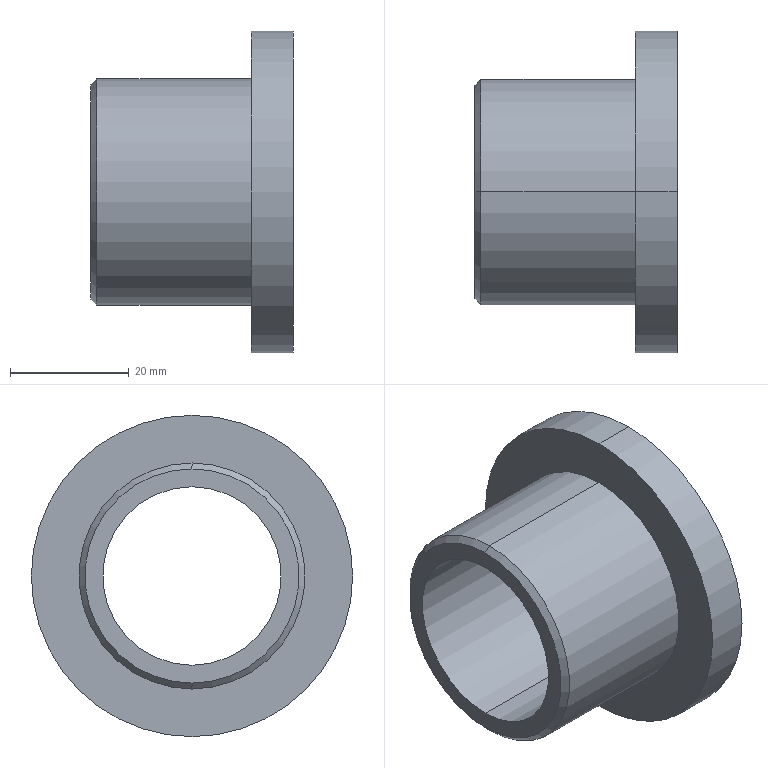Part | SolidWorks | features Chamfer 1, Revolution 1 | 1 solid | 11 faces | box 34 x 54 x 54 mm | volume 22561 mm3 | cylinder 6 | plane 3 | cone 2 | commonest cylinder face diameters 30 x2 38 x2 54 x2
STEP:
#1=CARTESIAN_POINT('',(0.,0.,18.));
#2=VERTEX_POINT('',#1);
#3=CARTESIAN_POINT('',(0.,0.,-18.));
#4=VERTEX_POINT('',#3);
#5=CARTESIAN_POINT('',(0.,0.,0.));
#6=DIRECTION('',(-1.,0.,0.));
#7=DIRECTION('',(0.,0.,-1.));
#8=AXIS2_PLACEMENT_3D('',#5,#6,#7);
#9=CIRCLE('',#8,18.);
#10=EDGE_CURVE('',#2,#4,#9,.T.);
#11=ORIENTED_EDGE('',*,*,#10,.F.);
#12=CARTESIAN_POINT('',(1.,0.,19.));
#13=VERTEX_POINT('',#12);
#14=CARTESIAN_POINT('',(0.,0.,18.));
#15=DIRECTION('',(0.7071,0.,0.7071));
#16=VECTOR('',#15,1000.);
#17=LINE('',#14,#16);
#18=EDGE_CURVE('',#2,#13,#17,.T.);
#19=ORIENTED_EDGE('',*,*,#18,.T.);
#20=CARTESIAN_POINT('',(1.,0.,-19.));
#21=VERTEX_POINT('',#20);
#22=CARTESIAN_POINT('',(1.,0.,0.));
#23=DIRECTION('',(1.,0.,0.));
#24=DIRECTION('',(0.,0.,-1.));
#25=AXIS2_PLACEMENT_3D('',#22,#23,#24);
#26=CIRCLE('',#25,19.);
#27=EDGE_CURVE('',#21,#13,#26,.T.);
#28=ORIENTED_EDGE('',*,*,#27,.F.);
#29=CARTESIAN_POINT('',(0.,0.,-18.));
#30=DIRECTION('',(0.7071,0.,-0.7071));
#31=VECTOR('',#30,1000.);
#32=LINE('',#29,#31);
#33=EDGE_CURVE('',#4,#21,#32,.T.);
#34=ORIENTED_EDGE('',*,*,#33,.F.);
#35=EDGE_LOOP('',(#11,#19,#28,#34));
#36=FACE_OUTER_BOUND('',#35,.T.);
#37=CARTESIAN_POINT('',(0.,0.,0.));
#38=DIRECTION('',(1.,0.,0.));
#39=DIRECTION('',(0.,0.,-1.));
#40=AXIS2_PLACEMENT_3D('',#37,#38,#39);
#41=CONICAL_SURFACE('',#40,18.,0.7854);
#42=ADVANCED_FACE('',(#36),#41,.T.);
#43=CARTESIAN_POINT('',(27.,0.,19.));
#44=VERTEX_POINT('',#43);
#45=CARTESIAN_POINT('',(27.,0.,-19.));
#46=VERTEX_POINT('',#45);
#47=CARTESIAN_POINT('',(27.,0.,0.));
#48=DIRECTION('',(-1.,0.,0.));
#49=DIRECTION('',(0.,0.,1.));
#50=AXIS2_PLACEMENT_3D('',#47,#48,#49);
#51=CIRCLE('',#50,19.);
#52=EDGE_CURVE('',#44,#46,#51,.T.);
#53=ORIENTED_EDGE('',*,*,#52,.T.);
#54=CARTESIAN_POINT('',(0.,0.,-19.));
#55=DIRECTION('',(-1.,0.,0.));
#56=VECTOR('',#55,1000.);
#57=LINE('',#54,#56);
#58=EDGE_CURVE('',#46,#21,#57,.T.);
#59=ORIENTED_EDGE('',*,*,#58,.T.);
#60=ORIENTED_EDGE('',*,*,#27,.T.);
#61=CARTESIAN_POINT('',(0.,0.,19.));
#62=DIRECTION('',(-1.,0.,0.));
#63=VECTOR('',#62,1000.);
#64=LINE('',#61,#63);
#65=EDGE_CURVE('',#44,#13,#64,.T.);
#66=ORIENTED_EDGE('',*,*,#65,.F.);
#67=EDGE_LOOP('',(#53,#59,#60,#66));
#68=FACE_OUTER_BOUND('',#67,.T.);
#69=CARTESIAN_POINT('',(0.,0.,0.));
#70=DIRECTION('',(-1.,0.,0.));
#71=DIRECTION('',(0.,0.,1.));
#72=AXIS2_PLACEMENT_3D('',#69,#70,#71);
#73=CYLINDRICAL_SURFACE('',#72,19.);
#74=ADVANCED_FACE('',(#68),#73,.T.);
#75=CARTESIAN_POINT('',(34.,0.,27.));
#76=VERTEX_POINT('',#75);
#77=CARTESIAN_POINT('',(34.,0.,-27.));
#78=VERTEX_POINT('',#77);
#79=CARTESIAN_POINT('',(34.,0.,0.));
#80=DIRECTION('',(-1.,0.,0.));
#81=DIRECTION('',(0.,0.,1.));
#82=AXIS2_PLACEMENT_3D('',#79,#80,#81);
#83=CIRCLE('',#82,27.);
#84=EDGE_CURVE('',#76,#78,#83,.T.);
#85=ORIENTED_EDGE('',*,*,#84,.T.);
#86=CARTESIAN_POINT('',(27.,0.,-27.));
#87=VERTEX_POINT('',#86);
#88=CARTESIAN_POINT('',(0.,0.,-27.));
#89=DIRECTION('',(-1.,0.,0.));
#90=VECTOR('',#89,1000.);
#91=LINE('',#88,#90);
#92=EDGE_CURVE('',#78,#87,#91,.T.);
#93=ORIENTED_EDGE('',*,*,#92,.T.);
#94=CARTESIAN_POINT('',(27.,0.,27.));
#95=VERTEX_POINT('',#94);
#96=CARTESIAN_POINT('',(27.,0.,0.));
#97=DIRECTION('',(-1.,0.,0.));
#98=DIRECTION('',(0.,0.,1.));
#99=AXIS2_PLACEMENT_3D('',#96,#97,#98);
#100=CIRCLE('',#99,27.);
#101=EDGE_CURVE('',#95,#87,#100,.T.);
#102=ORIENTED_EDGE('',*,*,#101,.F.);
#103=CARTESIAN_POINT('',(0.,0.,27.));
#104=DIRECTION('',(-1.,0.,0.));
#105=VECTOR('',#104,1000.);
#106=LINE('',#103,#105);
#107=EDGE_CURVE('',#76,#95,#106,.T.);
#108=ORIENTED_EDGE('',*,*,#107,.F.);
#109=EDGE_LOOP('',(#85,#93,#102,#108));
#110=FACE_OUTER_BOUND('',#109,.T.);
#111=CARTESIAN_POINT('',(0.,0.,0.));
#112=DIRECTION('',(-1.,0.,0.));
#113=DIRECTION('',(0.,0.,1.));
#114=AXIS2_PLACEMENT_3D('',#111,#112,#113);
#115=CYLINDRICAL_SURFACE('',#114,27.);
#116=ADVANCED_FACE('',(#110),#115,.T.);
#117=CARTESIAN_POINT('',(34.,0.,-15.));
#118=VERTEX_POINT('',#117);
#119=CARTESIAN_POINT('',(34.,0.,15.));
#120=VERTEX_POINT('',#119);
#121=CARTESIAN_POINT('',(34.,0.,0.));
#122=DIRECTION('',(-1.,0.,0.));
#123=DIRECTION('',(0.,0.,1.));
#124=AXIS2_PLACEMENT_3D('',#121,#122,#123);
#125=CIRCLE('',#124,15.);
#126=EDGE_CURVE('',#118,#120,#125,.T.);
#127=ORIENTED_EDGE('',*,*,#126,.F.);
#128=CARTESIAN_POINT('',(0.,0.,-15.));
#129=VERTEX_POINT('',#128);
#130=CARTESIAN_POINT('',(0.,0.,-15.));
#131=DIRECTION('',(-1.,0.,0.));
#132=VECTOR('',#131,1000.);
#133=LINE('',#130,#132);
#134=EDGE_CURVE('',#118,#129,#133,.T.);
#135=ORIENTED_EDGE('',*,*,#134,.T.);
#136=CARTESIAN_POINT('',(0.,0.,15.));
#137=VERTEX_POINT('',#136);
#138=CARTESIAN_POINT('',(0.,0.,0.));
#139=DIRECTION('',(-1.,0.,0.));
#140=DIRECTION('',(0.,0.,1.));
#141=AXIS2_PLACEMENT_3D('',#138,#139,#140);
#142=CIRCLE('',#141,15.);
#143=EDGE_CURVE('',#129,#137,#142,.T.);
#144=ORIENTED_EDGE('',*,*,#143,.T.);
#145=CARTESIAN_POINT('',(0.,0.,15.));
#146=DIRECTION('',(-1.,0.,0.));
#147=VECTOR('',#146,1000.);
#148=LINE('',#145,#147);
#149=EDGE_CURVE('',#120,#137,#148,.T.);
#150=ORIENTED_EDGE('',*,*,#149,.F.);
#151=EDGE_LOOP('',(#127,#135,#144,#150));
#152=FACE_OUTER_BOUND('',#151,.T.);
#153=CARTESIAN_POINT('',(0.,0.,0.));
#154=DIRECTION('',(-1.,0.,0.));
#155=DIRECTION('',(0.,0.,1.));
#156=AXIS2_PLACEMENT_3D('',#153,#154,#155);
#157=CYLINDRICAL_SURFACE('',#156,15.);
#158=ADVANCED_FACE('',(#152),#157,.F.);
#159=CARTESIAN_POINT('',(0.,0.,0.));
#160=DIRECTION('',(-1.,0.,0.));
#161=DIRECTION('',(0.,0.,-1.));
#162=AXIS2_PLACEMENT_3D('',#159,#160,#161);
#163=CIRCLE('',#162,18.);
#164=EDGE_CURVE('',#4,#2,#163,.T.);
#165=ORIENTED_EDGE('',*,*,#164,.T.);
#166=ORIENTED_EDGE('',*,*,#10,.T.);
#167=EDGE_LOOP('',(#165,#166));
#168=FACE_OUTER_BOUND('',#167,.T.);
#169=CARTESIAN_POINT('',(0.,0.,0.));
#170=DIRECTION('',(-1.,0.,0.));
#171=DIRECTION('',(0.,0.,1.));
#172=AXIS2_PLACEMENT_3D('',#169,#170,#171);
#173=CIRCLE('',#172,15.);
#174=EDGE_CURVE('',#137,#129,#173,.T.);
#175=ORIENTED_EDGE('',*,*,#174,.F.);
#176=ORIENTED_EDGE('',*,*,#143,.F.);
#177=EDGE_LOOP('',(#175,#176));
#178=FACE_BOUND('',#177,.T.);
#179=CARTESIAN_POINT('',(0.,19.,0.));
#180=DIRECTION('',(1.,0.,0.));
#181=DIRECTION('',(0.,0.,-1.));
#182=AXIS2_PLACEMENT_3D('',#179,#180,#181);
#183=PLANE('',#182);
#184=ADVANCED_FACE('',(#168,#178),#183,.F.);
#185=ORIENTED_EDGE('',*,*,#134,.F.);
#186=CARTESIAN_POINT('',(34.,0.,0.));
#187=DIRECTION('',(-1.,0.,0.));
#188=DIRECTION('',(0.,0.,1.));
#189=AXIS2_PLACEMENT_3D('',#186,#187,#188);
#190=CIRCLE('',#189,15.);
#191=EDGE_CURVE('',#120,#118,#190,.T.);
#192=ORIENTED_EDGE('',*,*,#191,.F.);
#193=ORIENTED_EDGE('',*,*,#149,.T.);
#194=ORIENTED_EDGE('',*,*,#174,.T.);
#195=EDGE_LOOP('',(#185,#192,#193,#194));
#196=FACE_OUTER_BOUND('',#195,.T.);
#197=CARTESIAN_POINT('',(0.,0.,0.));
#198=DIRECTION('',(-1.,0.,0.));
#199=DIRECTION('',(0.,0.,1.));
#200=AXIS2_PLACEMENT_3D('',#197,#198,#199);
#201=CYLINDRICAL_SURFACE('',#200,15.);
#202=ADVANCED_FACE('',(#196),#201,.F.);
#203=ORIENTED_EDGE('',*,*,#84,.F.);
#204=CARTESIAN_POINT('',(34.,0.,0.));
#205=DIRECTION('',(-1.,0.,0.));
#206=DIRECTION('',(0.,0.,1.));
#207=AXIS2_PLACEMENT_3D('',#204,#205,#206);
#208=CIRCLE('',#207,27.);
#209=EDGE_CURVE('',#78,#76,#208,.T.);
#210=ORIENTED_EDGE('',*,*,#209,.F.);
#211=EDGE_LOOP('',(#203,#210));
#212=FACE_OUTER_BOUND('',#211,.T.);
#213=ORIENTED_EDGE('',*,*,#191,.T.);
#214=ORIENTED_EDGE('',*,*,#126,.T.);
#215=EDGE_LOOP('',(#213,#214));
#216=FACE_BOUND('',#215,.T.);
#217=CARTESIAN_POINT('',(34.,15.,0.));
#218=DIRECTION('',(-1.,0.,0.));
#219=DIRECTION('',(0.,0.,1.));
#220=AXIS2_PLACEMENT_3D('',#217,#218,#219);
#221=PLANE('',#220);
#222=ADVANCED_FACE('',(#212,#216),#221,.F.);
#223=ORIENTED_EDGE('',*,*,#92,.F.);
#224=ORIENTED_EDGE('',*,*,#209,.T.);
#225=ORIENTED_EDGE('',*,*,#107,.T.);
#226=CARTESIAN_POINT('',(27.,0.,0.));
#227=DIRECTION('',(-1.,0.,0.));
#228=DIRECTION('',(0.,0.,1.));
#229=AXIS2_PLACEMENT_3D('',#226,#227,#228);
#230=CIRCLE('',#229,27.);
#231=EDGE_CURVE('',#87,#95,#230,.T.);
#232=ORIENTED_EDGE('',*,*,#231,.F.);
#233=EDGE_LOOP('',(#223,#224,#225,#232));
#234=FACE_OUTER_BOUND('',#233,.T.);
#235=CARTESIAN_POINT('',(0.,0.,0.));
#236=DIRECTION('',(-1.,0.,0.));
#237=DIRECTION('',(0.,0.,1.));
#238=AXIS2_PLACEMENT_3D('',#235,#236,#237);
#239=CYLINDRICAL_SURFACE('',#238,27.);
#240=ADVANCED_FACE('',(#234),#239,.T.);
#241=ORIENTED_EDGE('',*,*,#52,.F.);
#242=CARTESIAN_POINT('',(27.,0.,0.));
#243=DIRECTION('',(-1.,0.,0.));
#244=DIRECTION('',(0.,0.,1.));
#245=AXIS2_PLACEMENT_3D('',#242,#243,#244);
#246=CIRCLE('',#245,19.);
#247=EDGE_CURVE('',#46,#44,#246,.T.);
#248=ORIENTED_EDGE('',*,*,#247,.F.);
#249=EDGE_LOOP('',(#241,#248));
#250=FACE_BOUND('',#249,.T.);
#251=ORIENTED_EDGE('',*,*,#101,.T.);
#252=ORIENTED_EDGE('',*,*,#231,.T.);
#253=EDGE_LOOP('',(#251,#252));
#254=FACE_OUTER_BOUND('',#253,.T.);
#255=CARTESIAN_POINT('',(27.,27.,0.));
#256=DIRECTION('',(1.,0.,0.));
#257=DIRECTION('',(0.,0.,-1.));
#258=AXIS2_PLACEMENT_3D('',#255,#256,#257);
#259=PLANE('',#258);
#260=ADVANCED_FACE('',(#250,#254),#259,.F.);
#261=ORIENTED_EDGE('',*,*,#58,.F.);
#262=ORIENTED_EDGE('',*,*,#247,.T.);
#263=ORIENTED_EDGE('',*,*,#65,.T.);
#264=CARTESIAN_POINT('',(1.,0.,0.));
#265=DIRECTION('',(1.,0.,0.));
#266=DIRECTION('',(0.,0.,-1.));
#267=AXIS2_PLACEMENT_3D('',#264,#265,#266);
#268=CIRCLE('',#267,19.);
#269=EDGE_CURVE('',#13,#21,#268,.T.);
#270=ORIENTED_EDGE('',*,*,#269,.T.);
#271=EDGE_LOOP('',(#261,#262,#263,#270));
#272=FACE_OUTER_BOUND('',#271,.T.);
#273=CARTESIAN_POINT('',(0.,0.,0.));
#274=DIRECTION('',(-1.,0.,0.));
#275=DIRECTION('',(0.,0.,1.));
#276=AXIS2_PLACEMENT_3D('',#273,#274,#275);
#277=CYLINDRICAL_SURFACE('',#276,19.);
#278=ADVANCED_FACE('',(#272),#277,.T.);
#279=ORIENTED_EDGE('',*,*,#18,.F.);
#280=ORIENTED_EDGE('',*,*,#164,.F.);
#281=ORIENTED_EDGE('',*,*,#33,.T.);
#282=ORIENTED_EDGE('',*,*,#269,.F.);
#283=EDGE_LOOP('',(#279,#280,#281,#282));
#284=FACE_OUTER_BOUND('',#283,.T.);
#285=CARTESIAN_POINT('',(0.,0.,0.));
#286=DIRECTION('',(1.,0.,0.));
#287=DIRECTION('',(0.,0.,-1.));
#288=AXIS2_PLACEMENT_3D('',#285,#286,#287);
#289=CONICAL_SURFACE('',#288,18.,0.7854);
#290=ADVANCED_FACE('',(#284),#289,.T.);
#291=CLOSED_SHELL('',(#42,#74,#116,#158,#184,#202,#222,#240,#260,#278,#290));
#292=MANIFOLD_SOLID_BREP('',#291);
#293=CARTESIAN_POINT('',(0.,0.,0.));
#294=DIRECTION('',(0.,0.,1.));
#295=DIRECTION('',(1.,0.,0.));
#296=AXIS2_PLACEMENT_3D('',#293,#294,#295);
#297=(LENGTH_UNIT()NAMED_UNIT(*)SI_UNIT(.MILLI.,.METRE.));
#298=UNCERTAINTY_MEASURE_WITH_UNIT(LENGTH_MEASURE(0.00001),#297,'','');
#299=(NAMED_UNIT(*)PLANE_ANGLE_UNIT()SI_UNIT($,.RADIAN.));
#300=(NAMED_UNIT(*)SI_UNIT($,.STERADIAN.)SOLID_ANGLE_UNIT());
#301=(GEOMETRIC_REPRESENTATION_CONTEXT(3)GLOBAL_UNCERTAINTY_ASSIGNED_CONTEXT((#298))GLOBAL_UNIT_ASSIGNED_CONTEXT((#297,#299,#300))REPRESENTATION_CONTEXT('',''));
#302=ADVANCED_BREP_SHAPE_REPRESENTATION('',(#292,#296),#301);